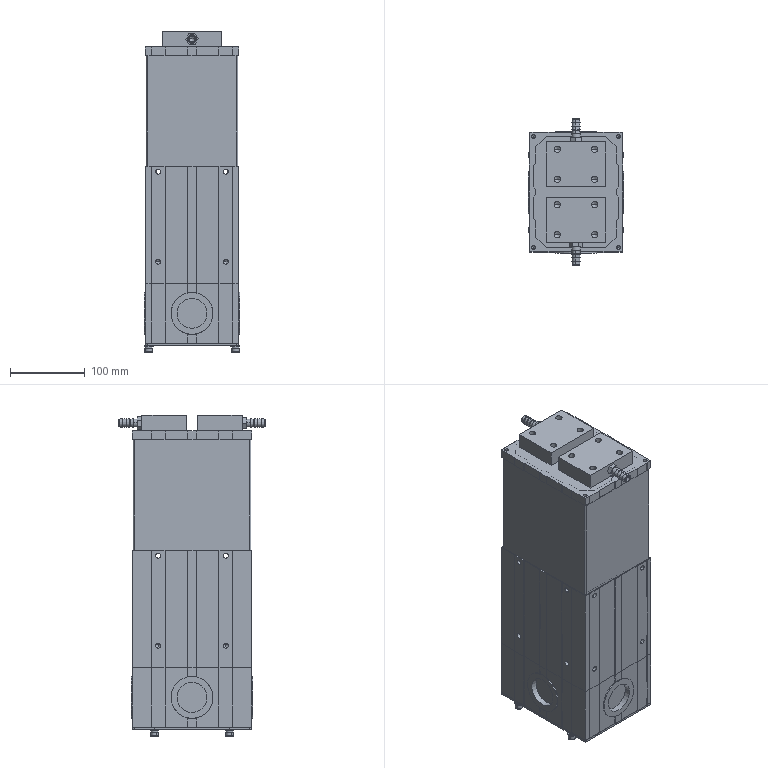Part | SolidWorks | features BaseBody 23 | 23 solids | 1245 faces | box 128 x 196 x 428.2 mm | volume 1860120 mm3 | plane 749 | cylinder 295 | cone 121 | spline 80 | commonest cylinder face diameters 5 x38 6.8 x32 6.6 x24 10 x24 56 x19 8.5 x18